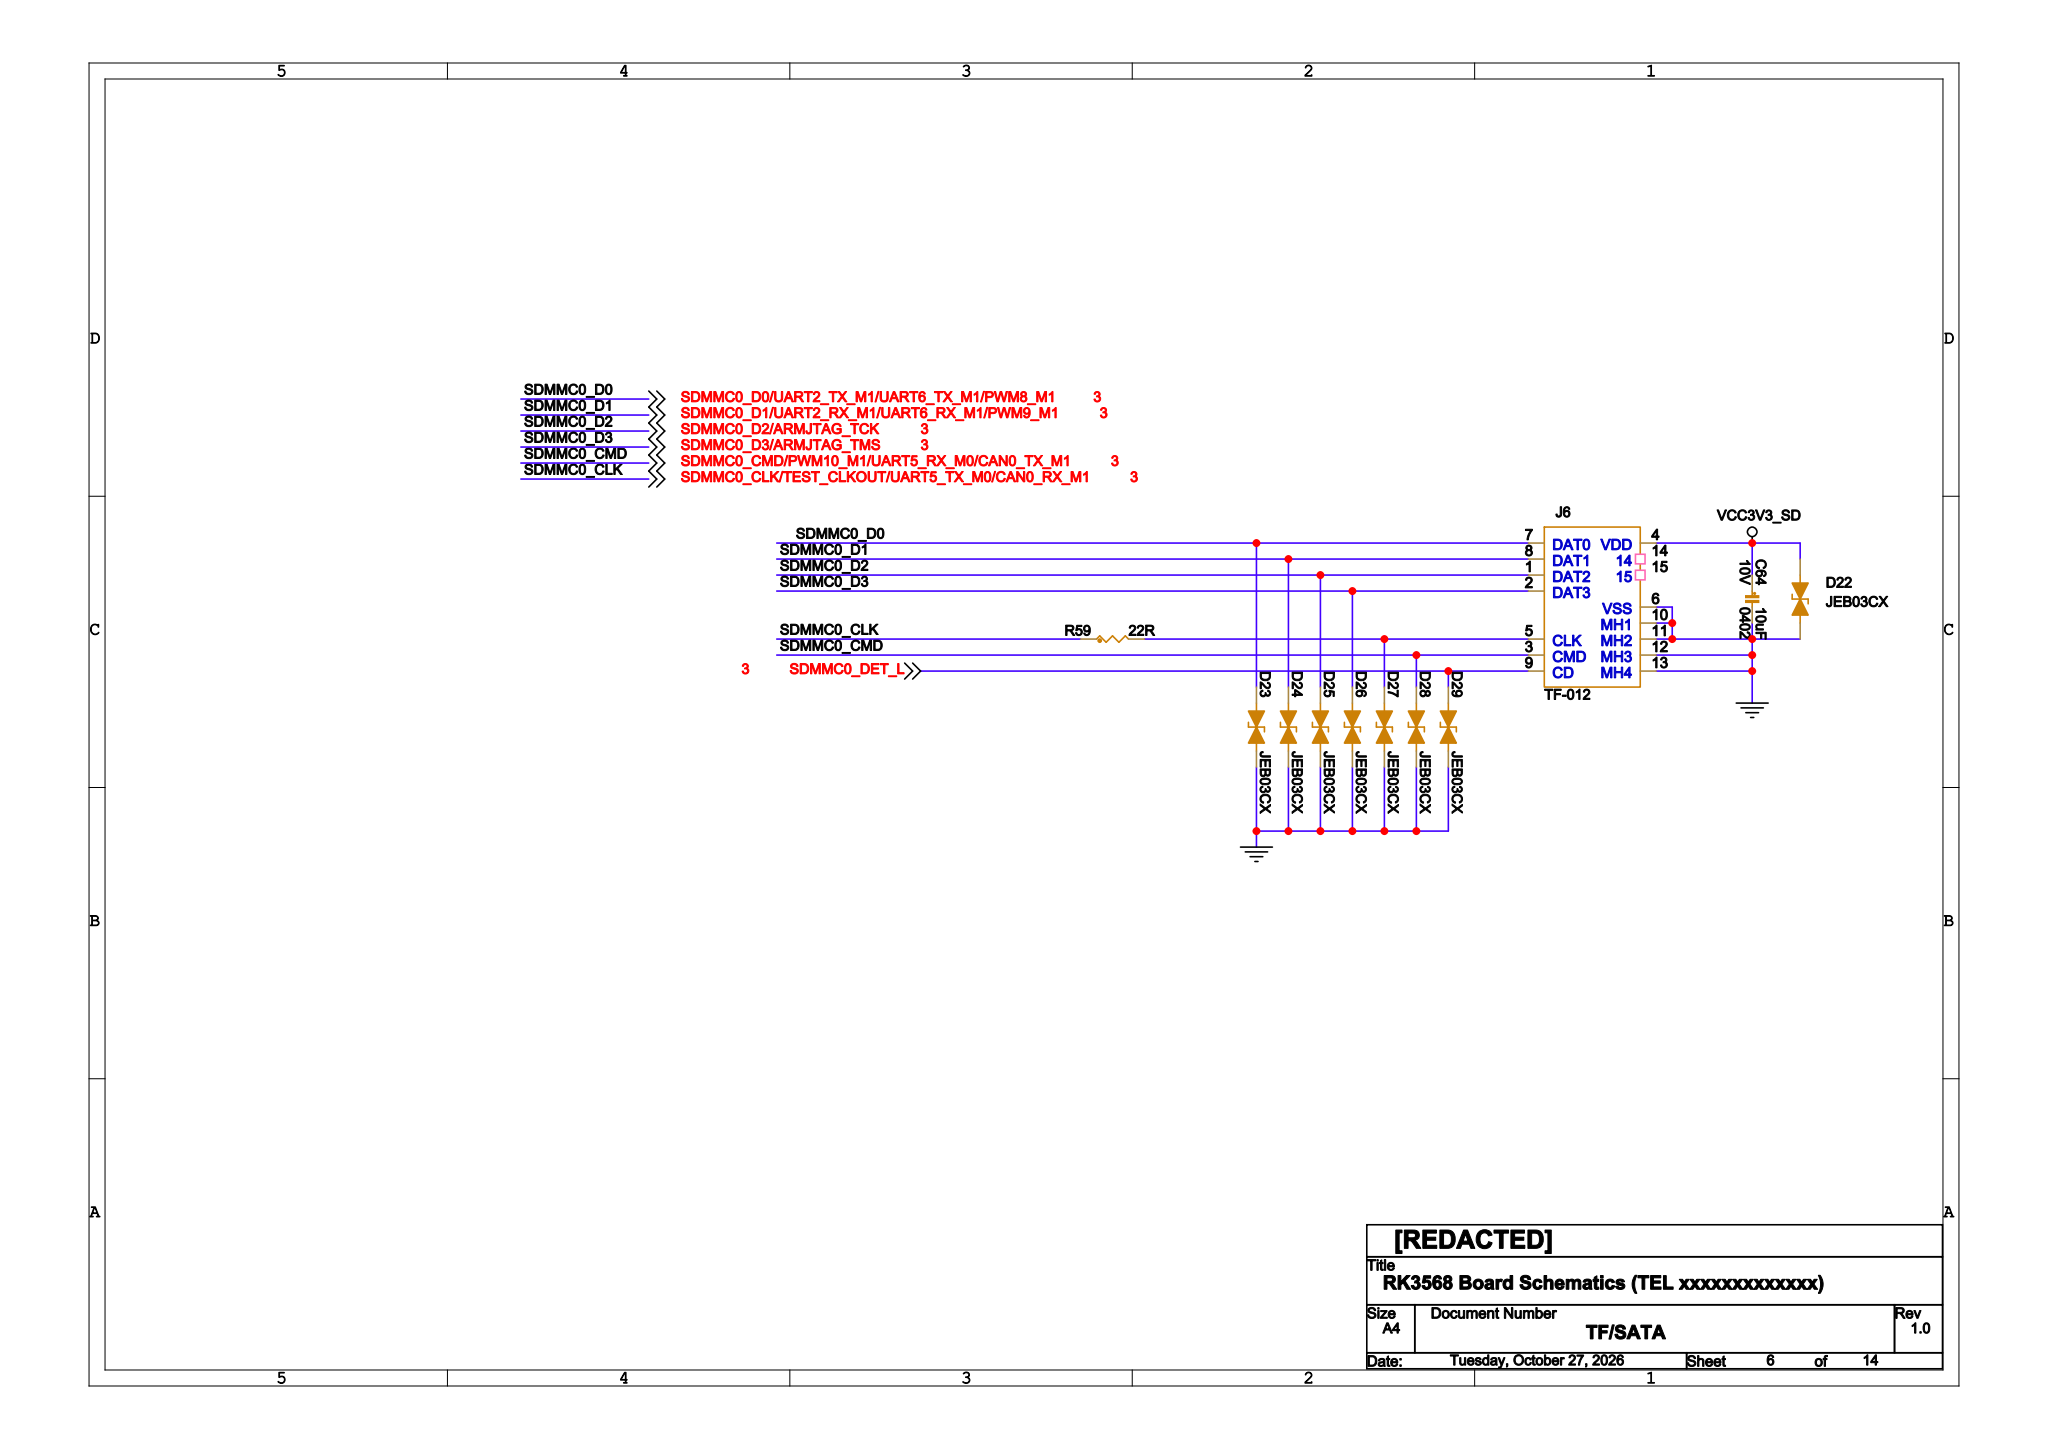Circuit board | Cadence Allegro | 669 parts | 581 nets | one sheet of the schematic
Parts on this sheet (reference | value | footprint):
C64 | 10uF | C0402
D22 | JEB03CX | SOD323
D23 | JEB03CX | SOD323
D24 | JEB03CX | SOD323
D25 | JEB03CX | SOD323
D26 | JEB03CX | SOD323
D27 | JEB03CX | SOD323
D28 | JEB03CX | SOD323
D29 | JEB03CX | SOD323
J6 | TF-012 | TFCARD1
R59 | 22R | R0402
Nets of these parts (net: part-pin ...):
GND: C64-2 D22-1 D23-1 D24-1 D25-1 D26-1 D27-1 D28-1 D29-1 J6-6 J6-10 J6-11 J6-12 J6-13
VCC3V3_SD: C64-1 D22-2 J6-4
SDMMC0_D0/UART2_TX_M1/UART6_TX_: D23-2 J6-7
SDMMC0_D1/UART2_RX_M1/UART6_RX_: D24-2 J6-8
SDMMC0_D2/ARMJTAG_TCK: D25-2 J6-1
SDMMC0_D3/ARMJTAG_TMS: D26-2 J6-2
N83883801: D27-2 J6-5 R59-2
SDMMC0_CMD/PWM10_M1/UART5_RX_M0: D28-2 J6-3
SDMMC0_DET_L: D29-2 J6-9
SDMMC0_CLK/TEST_CLKOUT/UART5_TX: R59-1